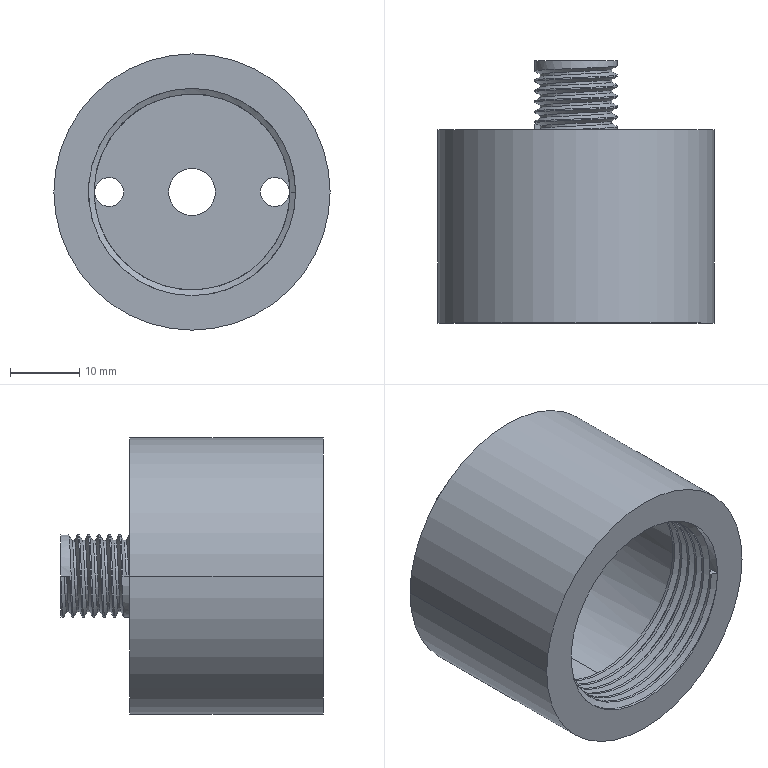Part | SolidWorks | features ICE 4, SweepThread 2, 3DProfileFeature 1, HoleWzd 1, Revolution 1 | 1 solid | 50 faces | box 40 x 38 x 40 mm | volume 19573 mm3 | cylinder 36 | plane 8 | spline 6 | commonest cylinder face diameters 12 x15 30 x13 4.2 x4 6.8 x2 40 x2